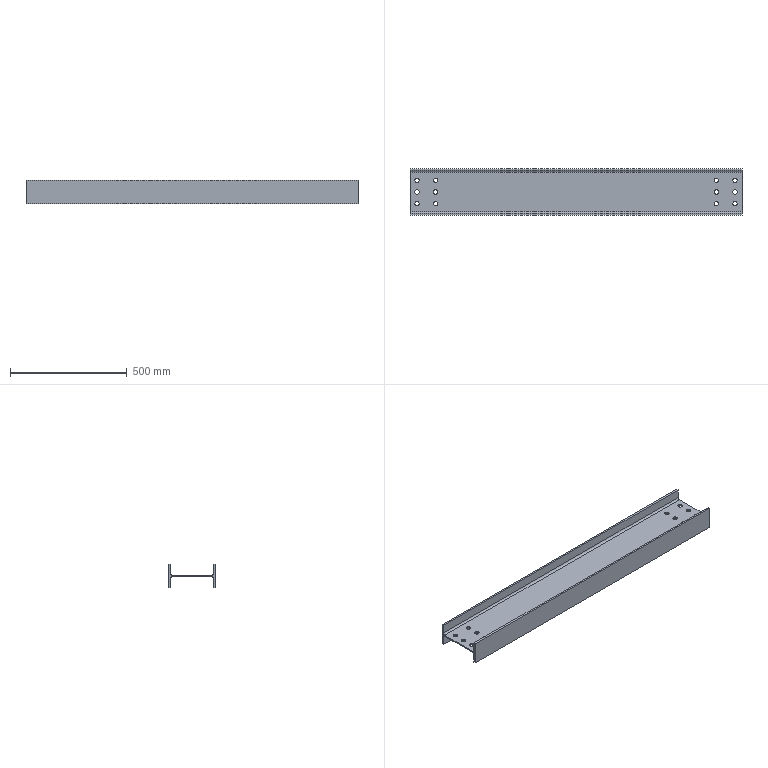Part | STEP file | 电柜主梁7主体_Default<As Machined> | 1 solid | 42 faces | box 1420 x 200 x 100 mm | volume 3768339 mm3 | cylinder 28 | plane 14 | commonest cylinder face diameters 19 x24 16 x4